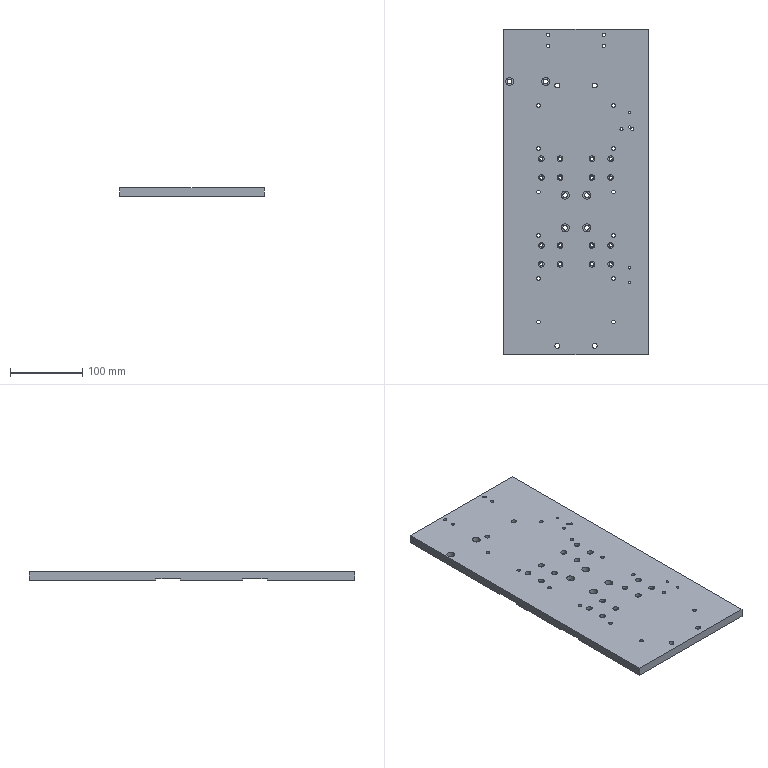Part | STEP file | PN_0040 Z-axis plate | 1 solid | 197 faces | box 200 x 450 x 12 mm | volume 1035466 mm3 | cylinder 152 | plane 41 | cone 4 | commonest cylinder face diameters 4.5 x40 8 x40 5 x28 6.6 x12 11 x12 3.3 x8